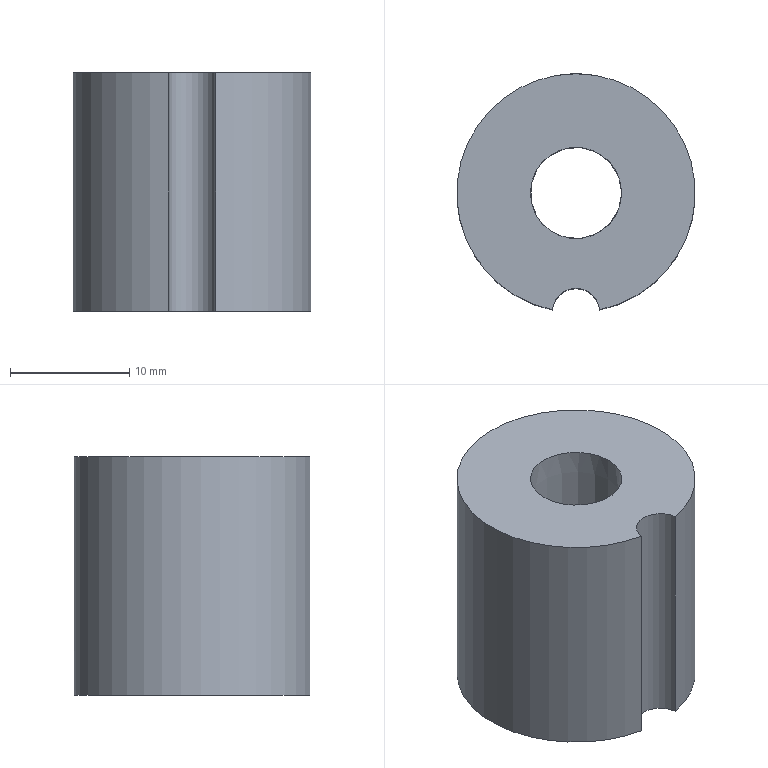Part | NX | features EKSD20-20-P7.66_2 2 | 1 solid | 199 faces | box 20 x 19.8 x 20 mm | volume 4295 mm3 | plane 111 | cylinder 87 | cone 1 | commonest cylinder face diameters 19.8 x15 20 x7 0.938 x3 0.48 x2 0.533 x2 0.537 x2